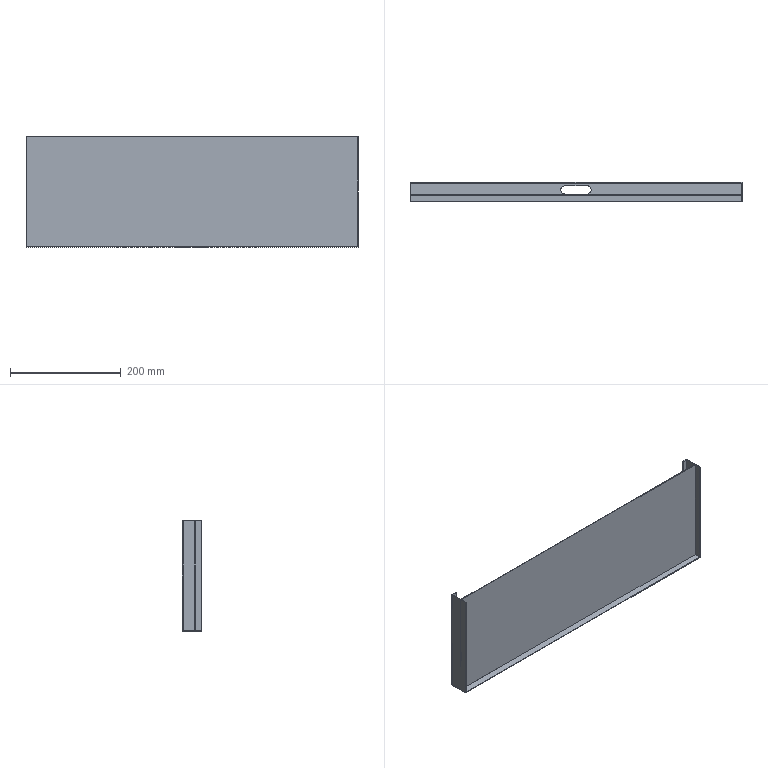Part | STEP file | Guide wheel mechanism revised.sldasm-Part-191 | 1 solid | 23 faces | box 600 x 35 x 200 mm | volume 241391 mm3 | plane 20 | cylinder 3 | commonest cylinder face diameters 15 x3
STEP:
#1=CARTESIAN_POINT('',(-20.,17.5,-98.5));
#2=VERTEX_POINT('',#1);
#3=CARTESIAN_POINT('',(-27.5,10.,-98.5));
#4=VERTEX_POINT('',#3);
#5=CARTESIAN_POINT('',(-20.,10.,-98.5));
#6=DIRECTION('',(0.,0.,1.));
#7=DIRECTION('',(-1.,0.,0.));
#8=AXIS2_PLACEMENT_3D('',#5,#6,#7);
#9=CIRCLE('',#8,7.5);
#10=EDGE_CURVE('',#2,#4,#9,.T.);
#11=ORIENTED_EDGE('',*,*,#10,.T.);
#12=CARTESIAN_POINT('',(-27.5,10.,-100.));
#13=VERTEX_POINT('',#12);
#14=CARTESIAN_POINT('',(-27.5,10.,130.001));
#15=DIRECTION('',(0.,0.,-1.));
#16=VECTOR('',#15,1000.);
#17=LINE('',#14,#16);
#18=EDGE_CURVE('',#4,#13,#17,.T.);
#19=ORIENTED_EDGE('',*,*,#18,.T.);
#20=CARTESIAN_POINT('',(-20.,17.5,-100.));
#21=VERTEX_POINT('',#20);
#22=CARTESIAN_POINT('',(-20.,10.,-100.));
#23=DIRECTION('',(0.,0.,-1.));
#24=DIRECTION('',(-1.,0.,0.));
#25=AXIS2_PLACEMENT_3D('',#22,#23,#24);
#26=CIRCLE('',#25,7.5);
#27=EDGE_CURVE('',#13,#21,#26,.T.);
#28=ORIENTED_EDGE('',*,*,#27,.T.);
#29=CARTESIAN_POINT('',(-20.,17.5,130.001));
#30=DIRECTION('',(0.,0.,-1.));
#31=VECTOR('',#30,1000.);
#32=LINE('',#29,#31);
#33=EDGE_CURVE('',#2,#21,#32,.T.);
#34=ORIENTED_EDGE('',*,*,#33,.F.);
#35=EDGE_LOOP('',(#11,#19,#28,#34));
#36=FACE_OUTER_BOUND('',#35,.T.);
#37=CARTESIAN_POINT('',(-20.,10.,130.001));
#38=DIRECTION('',(0.,0.,-1.));
#39=DIRECTION('',(-1.,0.,0.));
#40=AXIS2_PLACEMENT_3D('',#37,#38,#39);
#41=CYLINDRICAL_SURFACE('',#40,7.5);
#42=ADVANCED_FACE('',(#36),#41,.F.);
#43=CARTESIAN_POINT('',(298.5,1.5,100.));
#44=VERTEX_POINT('',#43);
#45=CARTESIAN_POINT('',(298.5,1.5,-98.5));
#46=VERTEX_POINT('',#45);
#47=CARTESIAN_POINT('',(298.5,1.5,100.));
#48=DIRECTION('',(0.,0.,-1.));
#49=VECTOR('',#48,1000.);
#50=LINE('',#47,#49);
#51=EDGE_CURVE('',#44,#46,#50,.T.);
#52=ORIENTED_EDGE('',*,*,#51,.T.);
#53=CARTESIAN_POINT('',(-298.5,1.5,-98.5));
#54=VERTEX_POINT('',#53);
#55=CARTESIAN_POINT('',(300.,1.5,-98.5));
#56=DIRECTION('',(-1.,0.,0.));
#57=VECTOR('',#56,1000.);
#58=LINE('',#55,#57);
#59=EDGE_CURVE('',#46,#54,#58,.T.);
#60=ORIENTED_EDGE('',*,*,#59,.T.);
#61=CARTESIAN_POINT('',(-298.5,1.5,100.));
#62=VERTEX_POINT('',#61);
#63=CARTESIAN_POINT('',(-298.5,1.5,100.));
#64=DIRECTION('',(0.,0.,1.));
#65=VECTOR('',#64,1000.);
#66=LINE('',#63,#65);
#67=EDGE_CURVE('',#54,#62,#66,.T.);
#68=ORIENTED_EDGE('',*,*,#67,.T.);
#69=CARTESIAN_POINT('',(-300.,1.5,100.));
#70=DIRECTION('',(1.,0.,0.));
#71=VECTOR('',#70,1000.);
#72=LINE('',#69,#71);
#73=EDGE_CURVE('',#62,#44,#72,.T.);
#74=ORIENTED_EDGE('',*,*,#73,.T.);
#75=EDGE_LOOP('',(#52,#60,#68,#74));
#76=FACE_OUTER_BOUND('',#75,.T.);
#77=CARTESIAN_POINT('',(300.,1.5,100.));
#78=DIRECTION('',(0.,1.,0.));
#79=DIRECTION('',(0.,0.,1.));
#80=AXIS2_PLACEMENT_3D('',#77,#78,#79);
#81=PLANE('',#80);
#82=ADVANCED_FACE('',(#76),#81,.T.);
#83=CARTESIAN_POINT('',(298.5,0.,-98.5));
#84=VERTEX_POINT('',#83);
#85=CARTESIAN_POINT('',(-298.5,0.,-98.5));
#86=VERTEX_POINT('',#85);
#87=CARTESIAN_POINT('',(300.,0.,-98.5));
#88=DIRECTION('',(-1.,0.,0.));
#89=VECTOR('',#88,1000.);
#90=LINE('',#87,#89);
#91=EDGE_CURVE('',#84,#86,#90,.T.);
#92=ORIENTED_EDGE('',*,*,#91,.F.);
#93=CARTESIAN_POINT('',(298.5,0.,100.));
#94=VERTEX_POINT('',#93);
#95=CARTESIAN_POINT('',(298.5,0.,100.));
#96=DIRECTION('',(0.,0.,-1.));
#97=VECTOR('',#96,1000.);
#98=LINE('',#95,#97);
#99=EDGE_CURVE('',#94,#84,#98,.T.);
#100=ORIENTED_EDGE('',*,*,#99,.F.);
#101=CARTESIAN_POINT('',(-298.5,0.,100.));
#102=VERTEX_POINT('',#101);
#103=CARTESIAN_POINT('',(-300.,0.,100.));
#104=DIRECTION('',(1.,0.,0.));
#105=VECTOR('',#104,1000.);
#106=LINE('',#103,#105);
#107=EDGE_CURVE('',#102,#94,#106,.T.);
#108=ORIENTED_EDGE('',*,*,#107,.F.);
#109=CARTESIAN_POINT('',(-298.5,0.,100.));
#110=DIRECTION('',(0.,0.,1.));
#111=VECTOR('',#110,1000.);
#112=LINE('',#109,#111);
#113=EDGE_CURVE('',#86,#102,#112,.T.);
#114=ORIENTED_EDGE('',*,*,#113,.F.);
#115=EDGE_LOOP('',(#92,#100,#108,#114));
#116=FACE_OUTER_BOUND('',#115,.T.);
#117=CARTESIAN_POINT('',(300.,0.,100.));
#118=DIRECTION('',(0.,1.,0.));
#119=DIRECTION('',(0.,0.,1.));
#120=AXIS2_PLACEMENT_3D('',#117,#118,#119);
#121=PLANE('',#120);
#122=ADVANCED_FACE('',(#116),#121,.F.);
#123=CARTESIAN_POINT('',(-298.5,-11.5,-98.5));
#124=VERTEX_POINT('',#123);
#125=CARTESIAN_POINT('',(-298.5,23.5,-98.5));
#126=DIRECTION('',(0.,-1.,0.));
#127=VECTOR('',#126,1000.);
#128=LINE('',#125,#127);
#129=EDGE_CURVE('',#86,#124,#128,.T.);
#130=ORIENTED_EDGE('',*,*,#129,.F.);
#131=ORIENTED_EDGE('',*,*,#113,.T.);
#132=CARTESIAN_POINT('',(-298.5,-11.5,100.));
#133=VERTEX_POINT('',#132);
#134=CARTESIAN_POINT('',(-298.5,-11.5,100.));
#135=DIRECTION('',(0.,1.,0.));
#136=VECTOR('',#135,1000.);
#137=LINE('',#134,#136);
#138=EDGE_CURVE('',#133,#102,#137,.T.);
#139=ORIENTED_EDGE('',*,*,#138,.F.);
#140=CARTESIAN_POINT('',(-298.5,-11.5,100.));
#141=DIRECTION('',(0.,0.,1.));
#142=VECTOR('',#141,1000.);
#143=LINE('',#140,#142);
#144=EDGE_CURVE('',#124,#133,#143,.T.);
#145=ORIENTED_EDGE('',*,*,#144,.F.);
#146=EDGE_LOOP('',(#130,#131,#139,#145));
#147=FACE_OUTER_BOUND('',#146,.T.);
#148=CARTESIAN_POINT('',(-298.5,23.5,100.));
#149=DIRECTION('',(-1.,0.,0.));
#150=DIRECTION('',(0.,0.,1.));
#151=AXIS2_PLACEMENT_3D('',#148,#149,#150);
#152=PLANE('',#151);
#153=ADVANCED_FACE('',(#147),#152,.F.);
#154=CARTESIAN_POINT('',(-298.5,22.,-98.5));
#155=VERTEX_POINT('',#154);
#156=CARTESIAN_POINT('',(-298.5,23.5,-98.5));
#157=DIRECTION('',(0.,-1.,0.));
#158=VECTOR('',#157,1000.);
#159=LINE('',#156,#158);
#160=EDGE_CURVE('',#155,#54,#159,.T.);
#161=ORIENTED_EDGE('',*,*,#160,.F.);
#162=CARTESIAN_POINT('',(-298.5,22.,100.));
#163=VERTEX_POINT('',#162);
#164=CARTESIAN_POINT('',(-298.5,22.,100.));
#165=DIRECTION('',(0.,0.,1.));
#166=VECTOR('',#165,1000.);
#167=LINE('',#164,#166);
#168=EDGE_CURVE('',#155,#163,#167,.T.);
#169=ORIENTED_EDGE('',*,*,#168,.T.);
#170=CARTESIAN_POINT('',(-298.5,-11.5,100.));
#171=DIRECTION('',(0.,1.,0.));
#172=VECTOR('',#171,1000.);
#173=LINE('',#170,#172);
#174=EDGE_CURVE('',#62,#163,#173,.T.);
#175=ORIENTED_EDGE('',*,*,#174,.F.);
#176=ORIENTED_EDGE('',*,*,#67,.F.);
#177=EDGE_LOOP('',(#161,#169,#175,#176));
#178=FACE_OUTER_BOUND('',#177,.T.);
#179=CARTESIAN_POINT('',(-298.5,23.5,100.));
#180=DIRECTION('',(-1.,0.,0.));
#181=DIRECTION('',(0.,0.,1.));
#182=AXIS2_PLACEMENT_3D('',#179,#180,#181);
#183=PLANE('',#182);
#184=ADVANCED_FACE('',(#178),#183,.F.);
#185=CARTESIAN_POINT('',(298.5,-11.5,-98.5));
#186=VERTEX_POINT('',#185);
#187=CARTESIAN_POINT('',(298.5,23.5,-98.5));
#188=DIRECTION('',(0.,1.,0.));
#189=VECTOR('',#188,1000.);
#190=LINE('',#187,#189);
#191=EDGE_CURVE('',#186,#84,#190,.T.);
#192=ORIENTED_EDGE('',*,*,#191,.F.);
#193=CARTESIAN_POINT('',(298.5,-11.5,100.));
#194=VERTEX_POINT('',#193);
#195=CARTESIAN_POINT('',(298.5,-11.5,100.));
#196=DIRECTION('',(0.,0.,1.));
#197=VECTOR('',#196,1000.);
#198=LINE('',#195,#197);
#199=EDGE_CURVE('',#186,#194,#198,.T.);
#200=ORIENTED_EDGE('',*,*,#199,.T.);
#201=CARTESIAN_POINT('',(298.5,-11.5,100.));
#202=DIRECTION('',(0.,1.,0.));
#203=VECTOR('',#202,1000.);
#204=LINE('',#201,#203);
#205=EDGE_CURVE('',#194,#94,#204,.T.);
#206=ORIENTED_EDGE('',*,*,#205,.T.);
#207=ORIENTED_EDGE('',*,*,#99,.T.);
#208=EDGE_LOOP('',(#192,#200,#206,#207));
#209=FACE_OUTER_BOUND('',#208,.T.);
#210=CARTESIAN_POINT('',(298.5,23.5,100.));
#211=DIRECTION('',(1.,0.,0.));
#212=DIRECTION('',(0.,0.,1.));
#213=AXIS2_PLACEMENT_3D('',#210,#211,#212);
#214=PLANE('',#213);
#215=ADVANCED_FACE('',(#209),#214,.F.);
#216=CARTESIAN_POINT('',(298.5,22.,100.));
#217=VERTEX_POINT('',#216);
#218=CARTESIAN_POINT('',(298.5,-11.5,100.));
#219=DIRECTION('',(0.,1.,0.));
#220=VECTOR('',#219,1000.);
#221=LINE('',#218,#220);
#222=EDGE_CURVE('',#44,#217,#221,.T.);
#223=ORIENTED_EDGE('',*,*,#222,.T.);
#224=CARTESIAN_POINT('',(298.5,22.,-98.5));
#225=VERTEX_POINT('',#224);
#226=CARTESIAN_POINT('',(298.5,22.,100.));
#227=DIRECTION('',(0.,0.,-1.));
#228=VECTOR('',#227,1000.);
#229=LINE('',#226,#228);
#230=EDGE_CURVE('',#217,#225,#229,.T.);
#231=ORIENTED_EDGE('',*,*,#230,.T.);
#232=CARTESIAN_POINT('',(298.5,23.5,-98.5));
#233=DIRECTION('',(0.,1.,0.));
#234=VECTOR('',#233,1000.);
#235=LINE('',#232,#234);
#236=EDGE_CURVE('',#46,#225,#235,.T.);
#237=ORIENTED_EDGE('',*,*,#236,.F.);
#238=ORIENTED_EDGE('',*,*,#51,.F.);
#239=EDGE_LOOP('',(#223,#231,#237,#238));
#240=FACE_OUTER_BOUND('',#239,.T.);
#241=CARTESIAN_POINT('',(298.5,23.5,100.));
#242=DIRECTION('',(1.,0.,0.));
#243=DIRECTION('',(0.,0.,1.));
#244=AXIS2_PLACEMENT_3D('',#241,#242,#243);
#245=PLANE('',#244);
#246=ADVANCED_FACE('',(#240),#245,.F.);
#247=CARTESIAN_POINT('',(300.,-11.5,-100.));
#248=VERTEX_POINT('',#247);
#249=CARTESIAN_POINT('',(300.,-11.5,100.));
#250=VERTEX_POINT('',#249);
#251=CARTESIAN_POINT('',(300.,-11.5,100.));
#252=DIRECTION('',(0.,0.,1.));
#253=VECTOR('',#252,1000.);
#254=LINE('',#251,#253);
#255=EDGE_CURVE('',#248,#250,#254,.T.);
#256=ORIENTED_EDGE('',*,*,#255,.F.);
#257=CARTESIAN_POINT('',(300.,23.5,-100.));
#258=VERTEX_POINT('',#257);
#259=CARTESIAN_POINT('',(300.,1.5,-100.));
#260=DIRECTION('',(0.,-1.,0.));
#261=VECTOR('',#260,1000.);
#262=LINE('',#259,#261);
#263=EDGE_CURVE('',#258,#248,#262,.T.);
#264=ORIENTED_EDGE('',*,*,#263,.F.);
#265=CARTESIAN_POINT('',(300.,23.5,100.));
#266=VERTEX_POINT('',#265);
#267=CARTESIAN_POINT('',(300.,23.5,100.));
#268=DIRECTION('',(0.,0.,-1.));
#269=VECTOR('',#268,1000.);
#270=LINE('',#267,#269);
#271=EDGE_CURVE('',#266,#258,#270,.T.);
#272=ORIENTED_EDGE('',*,*,#271,.F.);
#273=CARTESIAN_POINT('',(300.,1.5,100.));
#274=DIRECTION('',(0.,-1.,0.));
#275=VECTOR('',#274,1000.);
#276=LINE('',#273,#275);
#277=EDGE_CURVE('',#266,#250,#276,.T.);
#278=ORIENTED_EDGE('',*,*,#277,.T.);
#279=EDGE_LOOP('',(#256,#264,#272,#278));
#280=FACE_OUTER_BOUND('',#279,.T.);
#281=CARTESIAN_POINT('',(300.,1.5,-100.));
#282=DIRECTION('',(-1.,0.,0.));
#283=DIRECTION('',(0.,0.,1.));
#284=AXIS2_PLACEMENT_3D('',#281,#282,#283);
#285=PLANE('',#284);
#286=ADVANCED_FACE('',(#280),#285,.F.);
#287=CARTESIAN_POINT('',(20.,2.5,-100.));
#288=VERTEX_POINT('',#287);
#289=CARTESIAN_POINT('',(-20.,2.5,-100.));
#290=VERTEX_POINT('',#289);
#291=CARTESIAN_POINT('',(20.,2.5,-100.));
#292=DIRECTION('',(-1.,0.,0.));
#293=VECTOR('',#292,1000.);
#294=LINE('',#291,#293);
#295=EDGE_CURVE('',#288,#290,#294,.T.);
#296=ORIENTED_EDGE('',*,*,#295,.F.);
#297=CARTESIAN_POINT('',(20.,17.5,-100.));
#298=VERTEX_POINT('',#297);
#299=CARTESIAN_POINT('',(20.,10.,-100.));
#300=DIRECTION('',(0.,0.,-1.));
#301=DIRECTION('',(-1.,0.,0.));
#302=AXIS2_PLACEMENT_3D('',#299,#300,#301);
#303=CIRCLE('',#302,7.5);
#304=EDGE_CURVE('',#298,#288,#303,.T.);
#305=ORIENTED_EDGE('',*,*,#304,.F.);
#306=CARTESIAN_POINT('',(20.,17.5,-100.));
#307=DIRECTION('',(1.,0.,0.));
#308=VECTOR('',#307,1000.);
#309=LINE('',#306,#308);
#310=EDGE_CURVE('',#21,#298,#309,.T.);
#311=ORIENTED_EDGE('',*,*,#310,.F.);
#312=ORIENTED_EDGE('',*,*,#27,.F.);
#313=CARTESIAN_POINT('',(-20.,10.,-100.));
#314=DIRECTION('',(0.,0.,-1.));
#315=DIRECTION('',(-1.,0.,0.));
#316=AXIS2_PLACEMENT_3D('',#313,#314,#315);
#317=CIRCLE('',#316,7.5);
#318=EDGE_CURVE('',#290,#13,#317,.T.);
#319=ORIENTED_EDGE('',*,*,#318,.F.);
#320=EDGE_LOOP('',(#296,#305,#311,#312,#319));
#321=FACE_BOUND('',#320,.T.);
#322=CARTESIAN_POINT('',(-300.,-11.5,-100.));
#323=VERTEX_POINT('',#322);
#324=CARTESIAN_POINT('',(-298.5,-11.5,-100.));
#325=DIRECTION('',(-1.,0.,0.));
#326=VECTOR('',#325,1000.);
#327=LINE('',#324,#326);
#328=EDGE_CURVE('',#248,#323,#327,.T.);
#329=ORIENTED_EDGE('',*,*,#328,.T.);
#330=CARTESIAN_POINT('',(-300.,23.5,-100.));
#331=VERTEX_POINT('',#330);
#332=CARTESIAN_POINT('',(-300.,1.5,-100.));
#333=DIRECTION('',(0.,-1.,0.));
#334=VECTOR('',#333,1000.);
#335=LINE('',#332,#334);
#336=EDGE_CURVE('',#331,#323,#335,.T.);
#337=ORIENTED_EDGE('',*,*,#336,.F.);
#338=CARTESIAN_POINT('',(-298.5,23.5,-100.));
#339=DIRECTION('',(-1.,0.,0.));
#340=VECTOR('',#339,1000.);
#341=LINE('',#338,#340);
#342=EDGE_CURVE('',#258,#331,#341,.T.);
#343=ORIENTED_EDGE('',*,*,#342,.F.);
#344=ORIENTED_EDGE('',*,*,#263,.T.);
#345=EDGE_LOOP('',(#329,#337,#343,#344));
#346=FACE_OUTER_BOUND('',#345,.T.);
#347=CARTESIAN_POINT('',(-300.,1.5,-100.));
#348=DIRECTION('',(0.,0.,1.));
#349=DIRECTION('',(1.,0.,0.));
#350=AXIS2_PLACEMENT_3D('',#347,#348,#349);
#351=PLANE('',#350);
#352=ADVANCED_FACE('',(#321,#346),#351,.F.);
#353=CARTESIAN_POINT('',(-300.,-11.5,100.));
#354=VERTEX_POINT('',#353);
#355=CARTESIAN_POINT('',(-300.,-11.5,100.));
#356=DIRECTION('',(0.,0.,1.));
#357=VECTOR('',#356,1000.);
#358=LINE('',#355,#357);
#359=EDGE_CURVE('',#323,#354,#358,.T.);
#360=ORIENTED_EDGE('',*,*,#359,.T.);
#361=CARTESIAN_POINT('',(-300.,23.5,100.));
#362=VERTEX_POINT('',#361);
#363=CARTESIAN_POINT('',(-300.,1.5,100.));
#364=DIRECTION('',(0.,-1.,0.));
#365=VECTOR('',#364,1000.);
#366=LINE('',#363,#365);
#367=EDGE_CURVE('',#362,#354,#366,.T.);
#368=ORIENTED_EDGE('',*,*,#367,.F.);
#369=CARTESIAN_POINT('',(-300.,23.5,100.));
#370=DIRECTION('',(0.,0.,-1.));
#371=VECTOR('',#370,1000.);
#372=LINE('',#369,#371);
#373=EDGE_CURVE('',#362,#331,#372,.T.);
#374=ORIENTED_EDGE('',*,*,#373,.T.);
#375=ORIENTED_EDGE('',*,*,#336,.T.);
#376=EDGE_LOOP('',(#360,#368,#374,#375));
#377=FACE_OUTER_BOUND('',#376,.T.);
#378=CARTESIAN_POINT('',(-300.,1.5,-100.));
#379=DIRECTION('',(1.,0.,0.));
#380=DIRECTION('',(0.,0.,-1.));
#381=AXIS2_PLACEMENT_3D('',#378,#379,#380);
#382=PLANE('',#381);
#383=ADVANCED_FACE('',(#377),#382,.F.);
#384=CARTESIAN_POINT('',(298.5,-11.5,100.));
#385=DIRECTION('',(-1.,0.,0.));
#386=VECTOR('',#385,1000.);
#387=LINE('',#384,#386);
#388=EDGE_CURVE('',#250,#194,#387,.T.);
#389=ORIENTED_EDGE('',*,*,#388,.F.);
#390=ORIENTED_EDGE('',*,*,#277,.F.);
#391=CARTESIAN_POINT('',(290.,23.5,100.));
#392=VERTEX_POINT('',#391);
#393=CARTESIAN_POINT('',(298.5,23.5,100.));
#394=DIRECTION('',(-1.,0.,0.));
#395=VECTOR('',#394,1000.);
#396=LINE('',#393,#395);
#397=EDGE_CURVE('',#266,#392,#396,.T.);
#398=ORIENTED_EDGE('',*,*,#397,.T.);
#399=CARTESIAN_POINT('',(290.,22.,100.));
#400=VERTEX_POINT('',#399);
#401=CARTESIAN_POINT('',(290.,22.,100.));
#402=DIRECTION('',(0.,1.,0.));
#403=VECTOR('',#402,1000.);
#404=LINE('',#401,#403);
#405=EDGE_CURVE('',#400,#392,#404,.T.);
#406=ORIENTED_EDGE('',*,*,#405,.F.);
#407=CARTESIAN_POINT('',(300.,22.,100.));
#408=DIRECTION('',(1.,0.,0.));
#409=VECTOR('',#408,1000.);
#410=LINE('',#407,#409);
#411=EDGE_CURVE('',#400,#217,#410,.T.);
#412=ORIENTED_EDGE('',*,*,#411,.T.);
#413=ORIENTED_EDGE('',*,*,#222,.F.);
#414=ORIENTED_EDGE('',*,*,#73,.F.);
#415=ORIENTED_EDGE('',*,*,#174,.T.);
#416=CARTESIAN_POINT('',(-290.,22.,100.));
#417=VERTEX_POINT('',#416);
#418=CARTESIAN_POINT('',(-290.,22.,100.));
#419=DIRECTION('',(1.,0.,0.));
#420=VECTOR('',#419,1000.);
#421=LINE('',#418,#420);
#422=EDGE_CURVE('',#163,#417,#421,.T.);
#423=ORIENTED_EDGE('',*,*,#422,.T.);
#424=CARTESIAN_POINT('',(-290.,23.5,100.));
#425=VERTEX_POINT('',#424);
#426=CARTESIAN_POINT('',(-290.,22.,100.));
#427=DIRECTION('',(0.,1.,0.));
#428=VECTOR('',#427,1000.);
#429=LINE('',#426,#428);
#430=EDGE_CURVE('',#417,#425,#429,.T.);
#431=ORIENTED_EDGE('',*,*,#430,.T.);
#432=CARTESIAN_POINT('',(-298.5,23.5,100.));
#433=DIRECTION('',(-1.,0.,0.));
#434=VECTOR('',#433,1000.);
#435=LINE('',#432,#434);
#436=EDGE_CURVE('',#425,#362,#435,.T.);
#437=ORIENTED_EDGE('',*,*,#436,.T.);
#438=ORIENTED_EDGE('',*,*,#367,.T.);
#439=CARTESIAN_POINT('',(-298.5,-11.5,100.));
#440=DIRECTION('',(-1.,0.,0.));
#441=VECTOR('',#440,1000.);
#442=LINE('',#439,#441);
#443=EDGE_CURVE('',#133,#354,#442,.T.);
#444=ORIENTED_EDGE('',*,*,#443,.F.);
#445=ORIENTED_EDGE('',*,*,#138,.T.);
#446=ORIENTED_EDGE('',*,*,#107,.T.);
#447=ORIENTED_EDGE('',*,*,#205,.F.);
#448=EDGE_LOOP('',(#389,#390,#398,#406,#412,#413,#414,#415,#423,#431,#437,#438,#444,#445,#446,#447));
#449=FACE_OUTER_BOUND('',#448,.T.);
#450=CARTESIAN_POINT('',(-300.,1.5,100.));
#451=DIRECTION('',(0.,0.,-1.));
#452=DIRECTION('',(-1.,0.,0.));
#453=AXIS2_PLACEMENT_3D('',#450,#451,#452);
#454=PLANE('',#453);
#455=ADVANCED_FACE('',(#449),#454,.F.);
#456=CARTESIAN_POINT('',(300.,-11.5,-98.5));
#457=DIRECTION('',(-1.,0.,0.));
#458=VECTOR('',#457,1000.);
#459=LINE('',#456,#458);
#460=EDGE_CURVE('',#186,#124,#459,.T.);
#461=ORIENTED_EDGE('',*,*,#460,.T.);
#462=ORIENTED_EDGE('',*,*,#144,.T.);
#463=ORIENTED_EDGE('',*,*,#443,.T.);
#464=ORIENTED_EDGE('',*,*,#359,.F.);
#465=ORIENTED_EDGE('',*,*,#328,.F.);
#466=ORIENTED_EDGE('',*,*,#255,.T.);
#467=ORIENTED_EDGE('',*,*,#388,.T.);
#468=ORIENTED_EDGE('',*,*,#199,.F.);
#469=EDGE_LOOP('',(#461,#462,#463,#464,#465,#466,#467,#468));
#470=FACE_OUTER_BOUND('',#469,.T.);
#471=CARTESIAN_POINT('',(-298.5,-11.5,100.));
#472=DIRECTION('',(0.,-1.,0.));
#473=DIRECTION('',(0.,0.,-1.));
#474=AXIS2_PLACEMENT_3D('',#471,#472,#473);
#475=PLANE('',#474);
#476=ADVANCED_FACE('',(#470),#475,.T.);
#477=ORIENTED_EDGE('',*,*,#342,.T.);
#478=ORIENTED_EDGE('',*,*,#373,.F.);
#479=ORIENTED_EDGE('',*,*,#436,.F.);
#480=CARTESIAN_POINT('',(-290.,23.5,-90.));
#481=VERTEX_POINT('',#480);
#482=CARTESIAN_POINT('',(-290.,23.5,-90.));
#483=DIRECTION('',(0.,0.,-1.));
#484=VECTOR('',#483,1000.);
#485=LINE('',#482,#484);
#486=EDGE_CURVE('',#425,#481,#485,.T.);
#487=ORIENTED_EDGE('',*,*,#486,.T.);
#488=CARTESIAN_POINT('',(290.,23.5,-90.));
#489=VERTEX_POINT('',#488);
#490=CARTESIAN_POINT('',(-290.,23.5,-90.));
#491=DIRECTION('',(1.,0.,0.));
#492=VECTOR('',#491,1000.);
#493=LINE('',#490,#492);
#494=EDGE_CURVE('',#481,#489,#493,.T.);
#495=ORIENTED_EDGE('',*,*,#494,.T.);
#496=CARTESIAN_POINT('',(290.,23.5,-90.));
#497=DIRECTION('',(0.,0.,1.));
#498=VECTOR('',#497,1000.);
#499=LINE('',#496,#498);
#500=EDGE_CURVE('',#489,#392,#499,.T.);
#501=ORIENTED_EDGE('',*,*,#500,.T.);
#502=ORIENTED_EDGE('',*,*,#397,.F.);
#503=ORIENTED_EDGE('',*,*,#271,.T.);
#504=EDGE_LOOP('',(#477,#478,#479,#487,#495,#501,#502,#503));
#505=FACE_OUTER_BOUND('',#504,.T.);
#506=CARTESIAN_POINT('',(-298.5,23.5,100.));
#507=DIRECTION('',(0.,1.,0.));
#508=DIRECTION('',(0.,0.,1.));
#509=AXIS2_PLACEMENT_3D('',#506,#507,#508);
#510=PLANE('',#509);
#511=ADVANCED_FACE('',(#505),#510,.T.);
#512=CARTESIAN_POINT('',(20.,17.5,-98.5));
#513=VERTEX_POINT('',#512);
#514=CARTESIAN_POINT('',(20.,17.5,-98.5));
#515=DIRECTION('',(-1.,0.,0.));
#516=VECTOR('',#515,1000.);
#517=LINE('',#514,#516);
#518=EDGE_CURVE('',#513,#2,#517,.T.);
#519=ORIENTED_EDGE('',*,*,#518,.F.);
#520=CARTESIAN_POINT('',(20.,2.5,-98.5));
#521=VERTEX_POINT('',#520);
#522=CARTESIAN_POINT('',(20.,10.,-98.5));
#523=DIRECTION('',(0.,0.,1.));
#524=DIRECTION('',(-1.,0.,0.));
#525=AXIS2_PLACEMENT_3D('',#522,#523,#524);
#526=CIRCLE('',#525,7.5);
#527=EDGE_CURVE('',#521,#513,#526,.T.);
#528=ORIENTED_EDGE('',*,*,#527,.F.);
#529=CARTESIAN_POINT('',(-20.,2.5,-98.5));
#530=VERTEX_POINT('',#529);
#531=CARTESIAN_POINT('',(20.,2.5,-98.5));
#532=DIRECTION('',(1.,0.,0.));
#533=VECTOR('',#532,1000.);
#534=LINE('',#531,#533);
#535=EDGE_CURVE('',#530,#521,#534,.T.);
#536=ORIENTED_EDGE('',*,*,#535,.F.);
#537=CARTESIAN_POINT('',(-20.,10.,-98.5));
#538=DIRECTION('',(0.,0.,1.));
#539=DIRECTION('',(-1.,0.,0.));
#540=AXIS2_PLACEMENT_3D('',#537,#538,#539);
#541=CIRCLE('',#540,7.5);
#542=EDGE_CURVE('',#4,#530,#541,.T.);
#543=ORIENTED_EDGE('',*,*,#542,.F.);
#544=ORIENTED_EDGE('',*,*,#10,.F.);
#545=EDGE_LOOP('',(#519,#528,#536,#543,#544));
#546=FACE_BOUND('',#545,.T.);
#547=ORIENTED_EDGE('',*,*,#236,.T.);
#548=CARTESIAN_POINT('',(300.,22.,-98.5));
#549=DIRECTION('',(-1.,0.,0.));
#550=VECTOR('',#549,1000.);
#551=LINE('',#548,#550);
#552=EDGE_CURVE('',#225,#155,#551,.T.);
#553=ORIENTED_EDGE('',*,*,#552,.T.);
#554=ORIENTED_EDGE('',*,*,#160,.T.);
#555=ORIENTED_EDGE('',*,*,#59,.F.);
#556=EDGE_LOOP('',(#547,#553,#554,#555));
#557=FACE_OUTER_BOUND('',#556,.T.);
#558=CARTESIAN_POINT('',(300.,-11.5,-98.5));
#559=DIRECTION('',(0.,0.,-1.));
#560=DIRECTION('',(-1.,0.,0.));
#561=AXIS2_PLACEMENT_3D('',#558,#559,#560);
#562=PLANE('',#561);
#563=ADVANCED_FACE('',(#546,#557),#562,.F.);
#564=ORIENTED_EDGE('',*,*,#91,.T.);
#565=ORIENTED_EDGE('',*,*,#129,.T.);
#566=ORIENTED_EDGE('',*,*,#460,.F.);
#567=ORIENTED_EDGE('',*,*,#191,.T.);
#568=EDGE_LOOP('',(#564,#565,#566,#567));
#569=FACE_OUTER_BOUND('',#568,.T.);
#570=CARTESIAN_POINT('',(300.,-11.5,-98.5));
#571=DIRECTION('',(0.,0.,-1.));
#572=DIRECTION('',(-1.,0.,0.));
#573=AXIS2_PLACEMENT_3D('',#570,#571,#572);
#574=PLANE('',#573);
#575=ADVANCED_FACE('',(#569),#574,.F.);
#576=ORIENTED_EDGE('',*,*,#168,.F.);
#577=ORIENTED_EDGE('',*,*,#552,.F.);
#578=ORIENTED_EDGE('',*,*,#230,.F.);
#579=ORIENTED_EDGE('',*,*,#411,.F.);
#580=CARTESIAN_POINT('',(290.,22.,-90.));
#581=VERTEX_POINT('',#580);
#582=CARTESIAN_POINT('',(290.,22.,-90.));
#583=DIRECTION('',(0.,0.,1.));
#584=VECTOR('',#583,1000.);
#585=LINE('',#582,#584);
#586=EDGE_CURVE('',#581,#400,#585,.T.);
#587=ORIENTED_EDGE('',*,*,#586,.F.);
#588=CARTESIAN_POINT('',(-290.,22.,-90.));
#589=VERTEX_POINT('',#588);
#590=CARTESIAN_POINT('',(-290.,22.,-90.));
#591=DIRECTION('',(1.,0.,0.));
#592=VECTOR('',#591,1000.);
#593=LINE('',#590,#592);
#594=EDGE_CURVE('',#589,#581,#593,.T.);
#595=ORIENTED_EDGE('',*,*,#594,.F.);
#596=CARTESIAN_POINT('',(-290.,22.,-90.));
#597=DIRECTION('',(0.,0.,-1.));
#598=VECTOR('',#597,1000.);
#599=LINE('',#596,#598);
#600=EDGE_CURVE('',#417,#589,#599,.T.);
#601=ORIENTED_EDGE('',*,*,#600,.F.);
#602=ORIENTED_EDGE('',*,*,#422,.F.);
#603=EDGE_LOOP('',(#576,#577,#578,#579,#587,#595,#601,#602));
#604=FACE_OUTER_BOUND('',#603,.T.);
#605=CARTESIAN_POINT('',(-300.,22.,100.));
#606=DIRECTION('',(0.,-1.,0.));
#607=DIRECTION('',(0.,0.,-1.));
#608=AXIS2_PLACEMENT_3D('',#605,#606,#607);
#609=PLANE('',#608);
#610=ADVANCED_FACE('',(#604),#609,.T.);
#611=ORIENTED_EDGE('',*,*,#500,.F.);
#612=CARTESIAN_POINT('',(290.,22.,-90.));
#613=DIRECTION('',(0.,1.,0.));
#614=VECTOR('',#613,1000.);
#615=LINE('',#612,#614);
#616=EDGE_CURVE('',#581,#489,#615,.T.);
#617=ORIENTED_EDGE('',*,*,#616,.F.);
#618=ORIENTED_EDGE('',*,*,#586,.T.);
#619=ORIENTED_EDGE('',*,*,#405,.T.);
#620=EDGE_LOOP('',(#611,#617,#618,#619));
#621=FACE_OUTER_BOUND('',#620,.T.);
#622=CARTESIAN_POINT('',(290.,22.,-90.));
#623=DIRECTION('',(-1.,0.,0.));
#624=DIRECTION('',(0.,0.,1.));
#625=AXIS2_PLACEMENT_3D('',#622,#623,#624);
#626=PLANE('',#625);
#627=ADVANCED_FACE('',(#621),#626,.T.);
#628=ORIENTED_EDGE('',*,*,#494,.F.);
#629=CARTESIAN_POINT('',(-290.,22.,-90.));
#630=DIRECTION('',(0.,1.,0.));
#631=VECTOR('',#630,1000.);
#632=LINE('',#629,#631);
#633=EDGE_CURVE('',#589,#481,#632,.T.);
#634=ORIENTED_EDGE('',*,*,#633,.F.);
#635=ORIENTED_EDGE('',*,*,#594,.T.);
#636=ORIENTED_EDGE('',*,*,#616,.T.);
#637=EDGE_LOOP('',(#628,#634,#635,#636));
#638=FACE_OUTER_BOUND('',#637,.T.);
#639=CARTESIAN_POINT('',(-290.,22.,-90.));
#640=DIRECTION('',(0.,0.,1.));
#641=DIRECTION('',(0.,-1.,0.));
#642=AXIS2_PLACEMENT_3D('',#639,#640,#641);
#643=PLANE('',#642);
#644=ADVANCED_FACE('',(#638),#643,.T.);
#645=ORIENTED_EDGE('',*,*,#486,.F.);
#646=ORIENTED_EDGE('',*,*,#430,.F.);
#647=ORIENTED_EDGE('',*,*,#600,.T.);
#648=ORIENTED_EDGE('',*,*,#633,.T.);
#649=EDGE_LOOP('',(#645,#646,#647,#648));
#650=FACE_OUTER_BOUND('',#649,.T.);
#651=CARTESIAN_POINT('',(-290.,22.,-90.));
#652=DIRECTION('',(1.,0.,0.));
#653=DIRECTION('',(0.,0.,-1.));
#654=AXIS2_PLACEMENT_3D('',#651,#652,#653);
#655=PLANE('',#654);
#656=ADVANCED_FACE('',(#650),#655,.T.);
#657=ORIENTED_EDGE('',*,*,#527,.T.);
#658=CARTESIAN_POINT('',(20.,17.5,130.001));
#659=DIRECTION('',(0.,0.,-1.));
#660=VECTOR('',#659,1000.);
#661=LINE('',#658,#660);
#662=EDGE_CURVE('',#513,#298,#661,.T.);
#663=ORIENTED_EDGE('',*,*,#662,.T.);
#664=ORIENTED_EDGE('',*,*,#304,.T.);
#665=CARTESIAN_POINT('',(20.,2.5,130.001));
#666=DIRECTION('',(0.,0.,-1.));
#667=VECTOR('',#666,1000.);
#668=LINE('',#665,#667);
#669=EDGE_CURVE('',#521,#288,#668,.T.);
#670=ORIENTED_EDGE('',*,*,#669,.F.);
#671=EDGE_LOOP('',(#657,#663,#664,#670));
#672=FACE_OUTER_BOUND('',#671,.T.);
#673=CARTESIAN_POINT('',(20.,10.,130.001));
#674=DIRECTION('',(0.,0.,-1.));
#675=DIRECTION('',(-1.,0.,0.));
#676=AXIS2_PLACEMENT_3D('',#673,#674,#675);
#677=CYLINDRICAL_SURFACE('',#676,7.5);
#678=ADVANCED_FACE('',(#672),#677,.F.);
#679=ORIENTED_EDGE('',*,*,#518,.T.);
#680=ORIENTED_EDGE('',*,*,#33,.T.);
#681=ORIENTED_EDGE('',*,*,#310,.T.);
#682=ORIENTED_EDGE('',*,*,#662,.F.);
#683=EDGE_LOOP('',(#679,#680,#681,#682));
#684=FACE_OUTER_BOUND('',#683,.T.);
#685=CARTESIAN_POINT('',(20.,17.5,130.001));
#686=DIRECTION('',(0.,1.,0.));
#687=DIRECTION('',(0.,0.,1.));
#688=AXIS2_PLACEMENT_3D('',#685,#686,#687);
#689=PLANE('',#688);
#690=ADVANCED_FACE('',(#684),#689,.F.);
#691=ORIENTED_EDGE('',*,*,#18,.F.);
#692=ORIENTED_EDGE('',*,*,#542,.T.);
#693=CARTESIAN_POINT('',(-20.,2.5,130.001));
#694=DIRECTION('',(0.,0.,-1.));
#695=VECTOR('',#694,1000.);
#696=LINE('',#693,#695);
#697=EDGE_CURVE('',#530,#290,#696,.T.);
#698=ORIENTED_EDGE('',*,*,#697,.T.);
#699=ORIENTED_EDGE('',*,*,#318,.T.);
#700=EDGE_LOOP('',(#691,#692,#698,#699));
#701=FACE_OUTER_BOUND('',#700,.T.);
#702=CARTESIAN_POINT('',(-20.,10.,130.001));
#703=DIRECTION('',(0.,0.,-1.));
#704=DIRECTION('',(-1.,0.,0.));
#705=AXIS2_PLACEMENT_3D('',#702,#703,#704);
#706=CYLINDRICAL_SURFACE('',#705,7.5);
#707=ADVANCED_FACE('',(#701),#706,.F.);
#708=ORIENTED_EDGE('',*,*,#535,.T.);
#709=ORIENTED_EDGE('',*,*,#669,.T.);
#710=ORIENTED_EDGE('',*,*,#295,.T.);
#711=ORIENTED_EDGE('',*,*,#697,.F.);
#712=EDGE_LOOP('',(#708,#709,#710,#711));
#713=FACE_OUTER_BOUND('',#712,.T.);
#714=CARTESIAN_POINT('',(20.,2.5,130.001));
#715=DIRECTION('',(0.,-1.,0.));
#716=DIRECTION('',(0.,0.,-1.));
#717=AXIS2_PLACEMENT_3D('',#714,#715,#716);
#718=PLANE('',#717);
#719=ADVANCED_FACE('',(#713),#718,.F.);
#720=CLOSED_SHELL('',(#42,#82,#122,#153,#184,#215,#246,#286,#352,#383,#455,#476,#511,#563,#575,#610,#627,#644,#656,#678,#690,#707,#719));
#721=MANIFOLD_SOLID_BREP('',#720);
#722=CARTESIAN_POINT('',(0.,0.,0.));
#723=DIRECTION('',(0.,0.,1.));
#724=DIRECTION('',(1.,0.,0.));
#725=AXIS2_PLACEMENT_3D('',#722,#723,#724);
#726=(LENGTH_UNIT()NAMED_UNIT(*)SI_UNIT(.MILLI.,.METRE.));
#727=UNCERTAINTY_MEASURE_WITH_UNIT(LENGTH_MEASURE(0.00001),#726,'','');
#728=(NAMED_UNIT(*)PLANE_ANGLE_UNIT()SI_UNIT($,.RADIAN.));
#729=(NAMED_UNIT(*)SI_UNIT($,.STERADIAN.)SOLID_ANGLE_UNIT());
#730=(GEOMETRIC_REPRESENTATION_CONTEXT(3)GLOBAL_UNCERTAINTY_ASSIGNED_CONTEXT((#727))GLOBAL_UNIT_ASSIGNED_CONTEXT((#726,#728,#729))REPRESENTATION_CONTEXT('',''));
#731=ADVANCED_BREP_SHAPE_REPRESENTATION('',(#721,#725),#730);